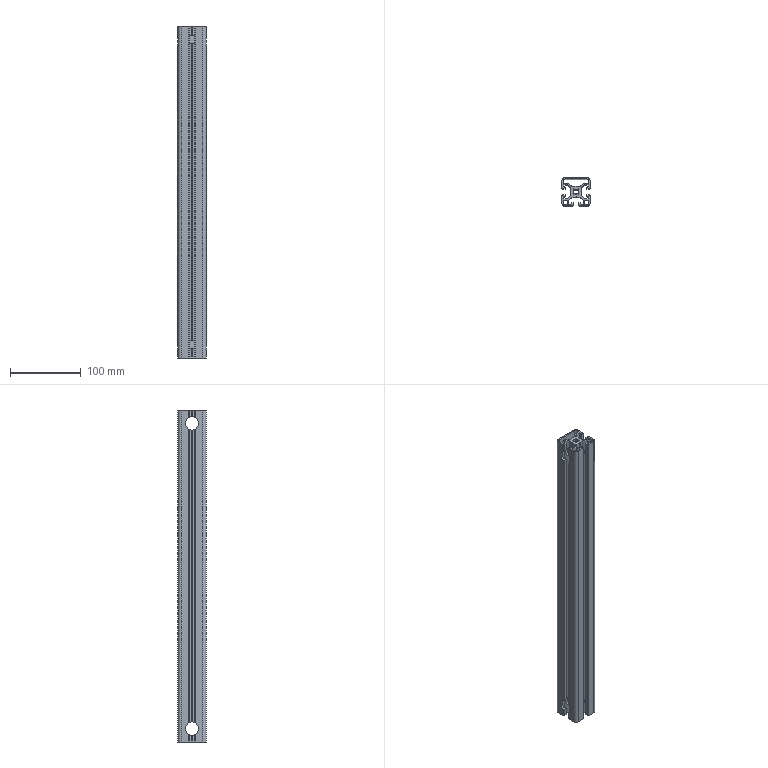Part | SolidWorks | features BaseBody 1, HoleWzd 1, MoveFace 1 | 1 solid | 242 faces | box 40 x 40 x 470 mm | volume 269890 mm3 | plane 187 | cylinder 55 | commonest cylinder face diameters 6.8 x15 2 x14 19 x12 1 x6 5 x4 9 x4